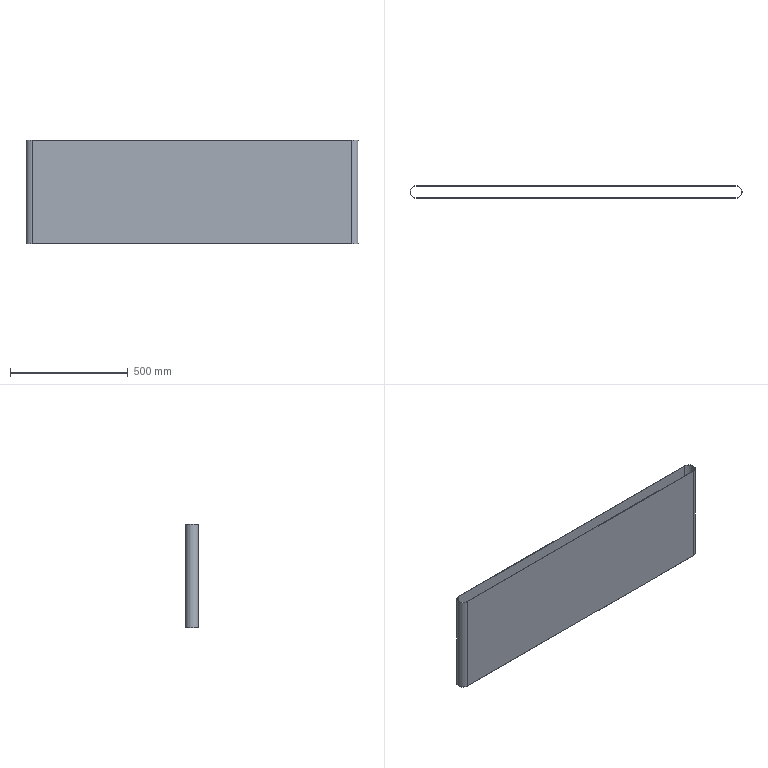Part | STEP file | RUBE 601 | 1 solid | 10 faces | box 1411 x 53.2 x 440 mm | volume 2026187 mm3 | plane 6 | cylinder 4 | commonest cylinder face diameters 50 x2 53.2 x2
STEP:
#1=CARTESIAN_POINT('',(0.,0.,0.));
#2=DIRECTION('',(0.,0.,1.));
#3=DIRECTION('',(1.,0.,0.));
#4=AXIS2_PLACEMENT_3D('',#1,#2,#3);
#5=CARTESIAN_POINT('',(-1248.5,28.6,220.));
#6=VERTEX_POINT('',#5);
#7=CARTESIAN_POINT('',(-1248.5,-24.6,220.));
#8=VERTEX_POINT('',#7);
#9=CARTESIAN_POINT('',(-1248.5,2.,220.));
#10=DIRECTION('',(0.,0.,1.));
#11=DIRECTION('',(1.,0.,0.));
#12=AXIS2_PLACEMENT_3D('',#9,#10,#11);
#13=CIRCLE('',#12,26.6);
#14=CARTESIAN_POINT('',(-1248.5,2.,220.));
#15=DIRECTION('',(0.,0.,1.));
#16=DIRECTION('',(1.,0.,0.));
#17=AXIS2_PLACEMENT_3D('',#14,#15,#16);
#18=PLANE('',#17);
#19=CARTESIAN_POINT('',(0.,0.));
#20=DIRECTION('',(1.,0.));
#21=AXIS2_PLACEMENT_2D('',#19,#20);
#22=CIRCLE('',#21,26.6);
#23=(GEOMETRIC_REPRESENTATION_CONTEXT(2)PARAMETRIC_REPRESENTATION_CONTEXT()REPRESENTATION_CONTEXT('',''));
#24=DEFINITIONAL_REPRESENTATION('',(#22),#23);
#25=PCURVE('',#18,#24);
#26=CARTESIAN_POINT('',(-1248.5,2.,220.));
#27=DIRECTION('',(0.,0.,-1.));
#28=DIRECTION('',(-1.,0.,0.));
#29=AXIS2_PLACEMENT_3D('',#26,#27,#28);
#30=CYLINDRICAL_SURFACE('',#29,26.6);
#31=CARTESIAN_POINT('',(3.142,0.));
#32=DIRECTION('',(-1.,0.));
#33=VECTOR('',#32,1.);
#34=LINE('',#31,#33);
#35=(GEOMETRIC_REPRESENTATION_CONTEXT(2)PARAMETRIC_REPRESENTATION_CONTEXT()REPRESENTATION_CONTEXT('',''));
#36=DEFINITIONAL_REPRESENTATION('',(#34),#35);
#37=PCURVE('',#30,#36);
#38=SURFACE_CURVE('',#13,(#25,#37),.PCURVE_S1.);
#39=EDGE_CURVE('',#6,#8,#38,.T.);
#40=ORIENTED_EDGE('',*,*,#39,.T.);
#41=CARTESIAN_POINT('',(109.5,-24.6,220.));
#42=VERTEX_POINT('',#41);
#43=CARTESIAN_POINT('',(-1248.5,-24.6,220.));
#44=DIRECTION('',(1.,0.,0.));
#45=VECTOR('',#44,1.);
#46=LINE('',#43,#45);
#47=CARTESIAN_POINT('',(0.,-26.6));
#48=DIRECTION('',(1.,0.));
#49=VECTOR('',#48,1.);
#50=LINE('',#47,#49);
#51=(GEOMETRIC_REPRESENTATION_CONTEXT(2)PARAMETRIC_REPRESENTATION_CONTEXT()REPRESENTATION_CONTEXT('',''));
#52=DEFINITIONAL_REPRESENTATION('',(#50),#51);
#53=PCURVE('',#18,#52);
#54=CARTESIAN_POINT('',(-1248.5,-24.6,220.));
#55=DIRECTION('',(0.,1.,0.));
#56=DIRECTION('',(-1.,0.,0.));
#57=AXIS2_PLACEMENT_3D('',#54,#55,#56);
#58=PLANE('',#57);
#59=CARTESIAN_POINT('',(0.,0.));
#60=DIRECTION('',(-1.,0.));
#61=VECTOR('',#60,1.);
#62=LINE('',#59,#61);
#63=(GEOMETRIC_REPRESENTATION_CONTEXT(2)PARAMETRIC_REPRESENTATION_CONTEXT()REPRESENTATION_CONTEXT('',''));
#64=DEFINITIONAL_REPRESENTATION('',(#62),#63);
#65=PCURVE('',#58,#64);
#66=SURFACE_CURVE('',#46,(#53,#65),.PCURVE_S1.);
#67=EDGE_CURVE('',#8,#42,#66,.T.);
#68=ORIENTED_EDGE('',*,*,#67,.T.);
#69=CARTESIAN_POINT('',(109.5,28.6,220.));
#70=VERTEX_POINT('',#69);
#71=CARTESIAN_POINT('',(109.5,2.,220.));
#72=DIRECTION('',(0.,0.,1.));
#73=DIRECTION('',(1.,0.,0.));
#74=AXIS2_PLACEMENT_3D('',#71,#72,#73);
#75=CIRCLE('',#74,26.6);
#76=CARTESIAN_POINT('',(1358.,0.));
#77=DIRECTION('',(1.,0.));
#78=AXIS2_PLACEMENT_2D('',#76,#77);
#79=CIRCLE('',#78,26.6);
#80=(GEOMETRIC_REPRESENTATION_CONTEXT(2)PARAMETRIC_REPRESENTATION_CONTEXT()REPRESENTATION_CONTEXT('',''));
#81=DEFINITIONAL_REPRESENTATION('',(#79),#80);
#82=PCURVE('',#18,#81);
#83=CARTESIAN_POINT('',(109.5,2.,220.));
#84=DIRECTION('',(0.,0.,-1.));
#85=DIRECTION('',(-1.,0.,0.));
#86=AXIS2_PLACEMENT_3D('',#83,#84,#85);
#87=CYLINDRICAL_SURFACE('',#86,26.6);
#88=CARTESIAN_POINT('',(9.425,0.));
#89=DIRECTION('',(-1.,0.));
#90=VECTOR('',#89,1.);
#91=LINE('',#88,#90);
#92=(GEOMETRIC_REPRESENTATION_CONTEXT(2)PARAMETRIC_REPRESENTATION_CONTEXT()REPRESENTATION_CONTEXT('',''));
#93=DEFINITIONAL_REPRESENTATION('',(#91),#92);
#94=PCURVE('',#87,#93);
#95=SURFACE_CURVE('',#75,(#82,#94),.PCURVE_S1.);
#96=EDGE_CURVE('',#42,#70,#95,.T.);
#97=ORIENTED_EDGE('',*,*,#96,.T.);
#98=CARTESIAN_POINT('',(-1248.5,28.6,220.));
#99=DIRECTION('',(-1.,0.,0.));
#100=VECTOR('',#99,1.);
#101=LINE('',#98,#100);
#102=CARTESIAN_POINT('',(0.,26.6));
#103=DIRECTION('',(-1.,0.));
#104=VECTOR('',#103,1.);
#105=LINE('',#102,#104);
#106=(GEOMETRIC_REPRESENTATION_CONTEXT(2)PARAMETRIC_REPRESENTATION_CONTEXT()REPRESENTATION_CONTEXT('',''));
#107=DEFINITIONAL_REPRESENTATION('',(#105),#106);
#108=PCURVE('',#18,#107);
#109=CARTESIAN_POINT('',(-1248.5,28.6,220.));
#110=DIRECTION('',(0.,-1.,0.));
#111=DIRECTION('',(1.,0.,0.));
#112=AXIS2_PLACEMENT_3D('',#109,#110,#111);
#113=PLANE('',#112);
#114=CARTESIAN_POINT('',(0.,0.));
#115=DIRECTION('',(-1.,0.));
#116=VECTOR('',#115,1.);
#117=LINE('',#114,#116);
#118=(GEOMETRIC_REPRESENTATION_CONTEXT(2)PARAMETRIC_REPRESENTATION_CONTEXT()REPRESENTATION_CONTEXT('',''));
#119=DEFINITIONAL_REPRESENTATION('',(#117),#118);
#120=PCURVE('',#113,#119);
#121=SURFACE_CURVE('',#101,(#108,#120),.PCURVE_S1.);
#122=EDGE_CURVE('',#70,#6,#121,.T.);
#123=ORIENTED_EDGE('',*,*,#122,.T.);
#124=EDGE_LOOP('',(#40,#68,#97,#123));
#125=FACE_BOUND('',#124,.T.);
#126=CARTESIAN_POINT('',(-1248.5,-23.,220.));
#127=VERTEX_POINT('',#126);
#128=CARTESIAN_POINT('',(109.5,-23.,220.));
#129=VERTEX_POINT('',#128);
#130=CARTESIAN_POINT('',(-1248.5,-23.,220.));
#131=DIRECTION('',(1.,0.,0.));
#132=VECTOR('',#131,1.);
#133=LINE('',#130,#132);
#134=CARTESIAN_POINT('',(0.,-25.));
#135=DIRECTION('',(1.,0.));
#136=VECTOR('',#135,1.);
#137=LINE('',#134,#136);
#138=(GEOMETRIC_REPRESENTATION_CONTEXT(2)PARAMETRIC_REPRESENTATION_CONTEXT()REPRESENTATION_CONTEXT('',''));
#139=DEFINITIONAL_REPRESENTATION('',(#137),#138);
#140=PCURVE('',#18,#139);
#141=CARTESIAN_POINT('',(-1248.5,-23.,220.));
#142=DIRECTION('',(0.,1.,0.));
#143=DIRECTION('',(-1.,0.,0.));
#144=AXIS2_PLACEMENT_3D('',#141,#142,#143);
#145=PLANE('',#144);
#146=CARTESIAN_POINT('',(0.,0.));
#147=DIRECTION('',(-1.,0.));
#148=VECTOR('',#147,1.);
#149=LINE('',#146,#148);
#150=(GEOMETRIC_REPRESENTATION_CONTEXT(2)PARAMETRIC_REPRESENTATION_CONTEXT()REPRESENTATION_CONTEXT('',''));
#151=DEFINITIONAL_REPRESENTATION('',(#149),#150);
#152=PCURVE('',#145,#151);
#153=SURFACE_CURVE('',#133,(#140,#152),.PCURVE_S1.);
#154=EDGE_CURVE('',#127,#129,#153,.T.);
#155=ORIENTED_EDGE('',*,*,#154,.F.);
#156=CARTESIAN_POINT('',(-1248.5,27.,220.));
#157=VERTEX_POINT('',#156);
#158=CARTESIAN_POINT('',(-1248.5,2.,220.));
#159=DIRECTION('',(0.,0.,1.));
#160=DIRECTION('',(1.,0.,0.));
#161=AXIS2_PLACEMENT_3D('',#158,#159,#160);
#162=CIRCLE('',#161,25.);
#163=CARTESIAN_POINT('',(0.,0.));
#164=DIRECTION('',(1.,0.));
#165=AXIS2_PLACEMENT_2D('',#163,#164);
#166=CIRCLE('',#165,25.);
#167=(GEOMETRIC_REPRESENTATION_CONTEXT(2)PARAMETRIC_REPRESENTATION_CONTEXT()REPRESENTATION_CONTEXT('',''));
#168=DEFINITIONAL_REPRESENTATION('',(#166),#167);
#169=PCURVE('',#18,#168);
#170=CARTESIAN_POINT('',(-1248.5,2.,220.));
#171=DIRECTION('',(0.,0.,-1.));
#172=DIRECTION('',(-1.,0.,0.));
#173=AXIS2_PLACEMENT_3D('',#170,#171,#172);
#174=CYLINDRICAL_SURFACE('',#173,25.);
#175=CARTESIAN_POINT('',(9.425,0.));
#176=DIRECTION('',(-1.,0.));
#177=VECTOR('',#176,1.);
#178=LINE('',#175,#177);
#179=(GEOMETRIC_REPRESENTATION_CONTEXT(2)PARAMETRIC_REPRESENTATION_CONTEXT()REPRESENTATION_CONTEXT('',''));
#180=DEFINITIONAL_REPRESENTATION('',(#178),#179);
#181=PCURVE('',#174,#180);
#182=SURFACE_CURVE('',#162,(#169,#181),.PCURVE_S1.);
#183=EDGE_CURVE('',#157,#127,#182,.T.);
#184=ORIENTED_EDGE('',*,*,#183,.F.);
#185=CARTESIAN_POINT('',(109.5,27.,220.));
#186=VERTEX_POINT('',#185);
#187=CARTESIAN_POINT('',(-1248.5,27.,220.));
#188=DIRECTION('',(-1.,0.,0.));
#189=VECTOR('',#188,1.);
#190=LINE('',#187,#189);
#191=CARTESIAN_POINT('',(0.,25.));
#192=DIRECTION('',(-1.,0.));
#193=VECTOR('',#192,1.);
#194=LINE('',#191,#193);
#195=(GEOMETRIC_REPRESENTATION_CONTEXT(2)PARAMETRIC_REPRESENTATION_CONTEXT()REPRESENTATION_CONTEXT('',''));
#196=DEFINITIONAL_REPRESENTATION('',(#194),#195);
#197=PCURVE('',#18,#196);
#198=CARTESIAN_POINT('',(-1248.5,27.,220.));
#199=DIRECTION('',(0.,-1.,0.));
#200=DIRECTION('',(1.,0.,0.));
#201=AXIS2_PLACEMENT_3D('',#198,#199,#200);
#202=PLANE('',#201);
#203=CARTESIAN_POINT('',(0.,0.));
#204=DIRECTION('',(-1.,0.));
#205=VECTOR('',#204,1.);
#206=LINE('',#203,#205);
#207=(GEOMETRIC_REPRESENTATION_CONTEXT(2)PARAMETRIC_REPRESENTATION_CONTEXT()REPRESENTATION_CONTEXT('',''));
#208=DEFINITIONAL_REPRESENTATION('',(#206),#207);
#209=PCURVE('',#202,#208);
#210=SURFACE_CURVE('',#190,(#197,#209),.PCURVE_S1.);
#211=EDGE_CURVE('',#186,#157,#210,.T.);
#212=ORIENTED_EDGE('',*,*,#211,.F.);
#213=CARTESIAN_POINT('',(109.5,2.,220.));
#214=DIRECTION('',(0.,0.,1.));
#215=DIRECTION('',(1.,0.,0.));
#216=AXIS2_PLACEMENT_3D('',#213,#214,#215);
#217=CIRCLE('',#216,25.);
#218=CARTESIAN_POINT('',(1358.,0.));
#219=DIRECTION('',(1.,0.));
#220=AXIS2_PLACEMENT_2D('',#218,#219);
#221=CIRCLE('',#220,25.);
#222=(GEOMETRIC_REPRESENTATION_CONTEXT(2)PARAMETRIC_REPRESENTATION_CONTEXT()REPRESENTATION_CONTEXT('',''));
#223=DEFINITIONAL_REPRESENTATION('',(#221),#222);
#224=PCURVE('',#18,#223);
#225=CARTESIAN_POINT('',(109.5,2.,220.));
#226=DIRECTION('',(0.,0.,-1.));
#227=DIRECTION('',(-1.,0.,0.));
#228=AXIS2_PLACEMENT_3D('',#225,#226,#227);
#229=CYLINDRICAL_SURFACE('',#228,25.);
#230=CARTESIAN_POINT('',(9.425,0.));
#231=DIRECTION('',(-1.,0.));
#232=VECTOR('',#231,1.);
#233=LINE('',#230,#232);
#234=(GEOMETRIC_REPRESENTATION_CONTEXT(2)PARAMETRIC_REPRESENTATION_CONTEXT()REPRESENTATION_CONTEXT('',''));
#235=DEFINITIONAL_REPRESENTATION('',(#233),#234);
#236=PCURVE('',#229,#235);
#237=SURFACE_CURVE('',#217,(#224,#236),.PCURVE_S1.);
#238=EDGE_CURVE('',#129,#186,#237,.T.);
#239=ORIENTED_EDGE('',*,*,#238,.F.);
#240=EDGE_LOOP('',(#155,#184,#212,#239));
#241=FACE_BOUND('',#240,.T.);
#242=ADVANCED_FACE('',(#125,#241),#18,.T.);
#243=CARTESIAN_POINT('',(-1248.5,28.6,-220.));
#244=VERTEX_POINT('',#243);
#245=CARTESIAN_POINT('',(-1248.5,-24.6,-220.));
#246=VERTEX_POINT('',#245);
#247=CARTESIAN_POINT('',(-1248.5,2.,-220.));
#248=DIRECTION('',(0.,0.,1.));
#249=DIRECTION('',(1.,0.,0.));
#250=AXIS2_PLACEMENT_3D('',#247,#248,#249);
#251=CIRCLE('',#250,26.6);
#252=CARTESIAN_POINT('',(-1248.5,2.,-220.));
#253=DIRECTION('',(0.,0.,1.));
#254=DIRECTION('',(1.,0.,0.));
#255=AXIS2_PLACEMENT_3D('',#252,#253,#254);
#256=PLANE('',#255);
#257=CARTESIAN_POINT('',(0.,0.));
#258=DIRECTION('',(1.,0.));
#259=AXIS2_PLACEMENT_2D('',#257,#258);
#260=CIRCLE('',#259,26.6);
#261=(GEOMETRIC_REPRESENTATION_CONTEXT(2)PARAMETRIC_REPRESENTATION_CONTEXT()REPRESENTATION_CONTEXT('',''));
#262=DEFINITIONAL_REPRESENTATION('',(#260),#261);
#263=PCURVE('',#256,#262);
#264=CARTESIAN_POINT('',(3.142,440.));
#265=DIRECTION('',(-1.,0.));
#266=VECTOR('',#265,1.);
#267=LINE('',#264,#266);
#268=(GEOMETRIC_REPRESENTATION_CONTEXT(2)PARAMETRIC_REPRESENTATION_CONTEXT()REPRESENTATION_CONTEXT('',''));
#269=DEFINITIONAL_REPRESENTATION('',(#267),#268);
#270=PCURVE('',#30,#269);
#271=SURFACE_CURVE('',#251,(#263,#270),.PCURVE_S1.);
#272=EDGE_CURVE('',#244,#246,#271,.T.);
#273=ORIENTED_EDGE('',*,*,#272,.F.);
#274=CARTESIAN_POINT('',(109.5,28.6,-220.));
#275=VERTEX_POINT('',#274);
#276=CARTESIAN_POINT('',(-1248.5,28.6,-220.));
#277=DIRECTION('',(-1.,0.,0.));
#278=VECTOR('',#277,1.);
#279=LINE('',#276,#278);
#280=CARTESIAN_POINT('',(0.,26.6));
#281=DIRECTION('',(-1.,0.));
#282=VECTOR('',#281,1.);
#283=LINE('',#280,#282);
#284=(GEOMETRIC_REPRESENTATION_CONTEXT(2)PARAMETRIC_REPRESENTATION_CONTEXT()REPRESENTATION_CONTEXT('',''));
#285=DEFINITIONAL_REPRESENTATION('',(#283),#284);
#286=PCURVE('',#256,#285);
#287=CARTESIAN_POINT('',(0.,-440.));
#288=DIRECTION('',(-1.,0.));
#289=VECTOR('',#288,1.);
#290=LINE('',#287,#289);
#291=(GEOMETRIC_REPRESENTATION_CONTEXT(2)PARAMETRIC_REPRESENTATION_CONTEXT()REPRESENTATION_CONTEXT('',''));
#292=DEFINITIONAL_REPRESENTATION('',(#290),#291);
#293=PCURVE('',#113,#292);
#294=SURFACE_CURVE('',#279,(#286,#293),.PCURVE_S1.);
#295=EDGE_CURVE('',#275,#244,#294,.T.);
#296=ORIENTED_EDGE('',*,*,#295,.F.);
#297=CARTESIAN_POINT('',(109.5,-24.6,-220.));
#298=VERTEX_POINT('',#297);
#299=CARTESIAN_POINT('',(109.5,2.,-220.));
#300=DIRECTION('',(0.,0.,1.));
#301=DIRECTION('',(1.,0.,0.));
#302=AXIS2_PLACEMENT_3D('',#299,#300,#301);
#303=CIRCLE('',#302,26.6);
#304=CARTESIAN_POINT('',(1358.,0.));
#305=DIRECTION('',(1.,0.));
#306=AXIS2_PLACEMENT_2D('',#304,#305);
#307=CIRCLE('',#306,26.6);
#308=(GEOMETRIC_REPRESENTATION_CONTEXT(2)PARAMETRIC_REPRESENTATION_CONTEXT()REPRESENTATION_CONTEXT('',''));
#309=DEFINITIONAL_REPRESENTATION('',(#307),#308);
#310=PCURVE('',#256,#309);
#311=CARTESIAN_POINT('',(9.425,440.));
#312=DIRECTION('',(-1.,0.));
#313=VECTOR('',#312,1.);
#314=LINE('',#311,#313);
#315=(GEOMETRIC_REPRESENTATION_CONTEXT(2)PARAMETRIC_REPRESENTATION_CONTEXT()REPRESENTATION_CONTEXT('',''));
#316=DEFINITIONAL_REPRESENTATION('',(#314),#315);
#317=PCURVE('',#87,#316);
#318=SURFACE_CURVE('',#303,(#310,#317),.PCURVE_S1.);
#319=EDGE_CURVE('',#298,#275,#318,.T.);
#320=ORIENTED_EDGE('',*,*,#319,.F.);
#321=CARTESIAN_POINT('',(-1248.5,-24.6,-220.));
#322=DIRECTION('',(1.,0.,0.));
#323=VECTOR('',#322,1.);
#324=LINE('',#321,#323);
#325=CARTESIAN_POINT('',(0.,-26.6));
#326=DIRECTION('',(1.,0.));
#327=VECTOR('',#326,1.);
#328=LINE('',#325,#327);
#329=(GEOMETRIC_REPRESENTATION_CONTEXT(2)PARAMETRIC_REPRESENTATION_CONTEXT()REPRESENTATION_CONTEXT('',''));
#330=DEFINITIONAL_REPRESENTATION('',(#328),#329);
#331=PCURVE('',#256,#330);
#332=CARTESIAN_POINT('',(0.,-440.));
#333=DIRECTION('',(-1.,0.));
#334=VECTOR('',#333,1.);
#335=LINE('',#332,#334);
#336=(GEOMETRIC_REPRESENTATION_CONTEXT(2)PARAMETRIC_REPRESENTATION_CONTEXT()REPRESENTATION_CONTEXT('',''));
#337=DEFINITIONAL_REPRESENTATION('',(#335),#336);
#338=PCURVE('',#58,#337);
#339=SURFACE_CURVE('',#324,(#331,#338),.PCURVE_S1.);
#340=EDGE_CURVE('',#246,#298,#339,.T.);
#341=ORIENTED_EDGE('',*,*,#340,.F.);
#342=EDGE_LOOP('',(#273,#296,#320,#341));
#343=FACE_BOUND('',#342,.T.);
#344=CARTESIAN_POINT('',(-1248.5,27.,-220.));
#345=VERTEX_POINT('',#344);
#346=CARTESIAN_POINT('',(-1248.5,-23.,-220.));
#347=VERTEX_POINT('',#346);
#348=CARTESIAN_POINT('',(-1248.5,2.,-220.));
#349=DIRECTION('',(0.,0.,1.));
#350=DIRECTION('',(1.,0.,0.));
#351=AXIS2_PLACEMENT_3D('',#348,#349,#350);
#352=CIRCLE('',#351,25.);
#353=CARTESIAN_POINT('',(0.,0.));
#354=DIRECTION('',(1.,0.));
#355=AXIS2_PLACEMENT_2D('',#353,#354);
#356=CIRCLE('',#355,25.);
#357=(GEOMETRIC_REPRESENTATION_CONTEXT(2)PARAMETRIC_REPRESENTATION_CONTEXT()REPRESENTATION_CONTEXT('',''));
#358=DEFINITIONAL_REPRESENTATION('',(#356),#357);
#359=PCURVE('',#256,#358);
#360=CARTESIAN_POINT('',(9.425,440.));
#361=DIRECTION('',(-1.,0.));
#362=VECTOR('',#361,1.);
#363=LINE('',#360,#362);
#364=(GEOMETRIC_REPRESENTATION_CONTEXT(2)PARAMETRIC_REPRESENTATION_CONTEXT()REPRESENTATION_CONTEXT('',''));
#365=DEFINITIONAL_REPRESENTATION('',(#363),#364);
#366=PCURVE('',#174,#365);
#367=SURFACE_CURVE('',#352,(#359,#366),.PCURVE_S1.);
#368=EDGE_CURVE('',#345,#347,#367,.T.);
#369=ORIENTED_EDGE('',*,*,#368,.T.);
#370=CARTESIAN_POINT('',(109.5,-23.,-220.));
#371=VERTEX_POINT('',#370);
#372=CARTESIAN_POINT('',(-1248.5,-23.,-220.));
#373=DIRECTION('',(1.,0.,0.));
#374=VECTOR('',#373,1.);
#375=LINE('',#372,#374);
#376=CARTESIAN_POINT('',(0.,-25.));
#377=DIRECTION('',(1.,0.));
#378=VECTOR('',#377,1.);
#379=LINE('',#376,#378);
#380=(GEOMETRIC_REPRESENTATION_CONTEXT(2)PARAMETRIC_REPRESENTATION_CONTEXT()REPRESENTATION_CONTEXT('',''));
#381=DEFINITIONAL_REPRESENTATION('',(#379),#380);
#382=PCURVE('',#256,#381);
#383=CARTESIAN_POINT('',(0.,-440.));
#384=DIRECTION('',(-1.,0.));
#385=VECTOR('',#384,1.);
#386=LINE('',#383,#385);
#387=(GEOMETRIC_REPRESENTATION_CONTEXT(2)PARAMETRIC_REPRESENTATION_CONTEXT()REPRESENTATION_CONTEXT('',''));
#388=DEFINITIONAL_REPRESENTATION('',(#386),#387);
#389=PCURVE('',#145,#388);
#390=SURFACE_CURVE('',#375,(#382,#389),.PCURVE_S1.);
#391=EDGE_CURVE('',#347,#371,#390,.T.);
#392=ORIENTED_EDGE('',*,*,#391,.T.);
#393=CARTESIAN_POINT('',(109.5,27.,-220.));
#394=VERTEX_POINT('',#393);
#395=CARTESIAN_POINT('',(109.5,2.,-220.));
#396=DIRECTION('',(0.,0.,1.));
#397=DIRECTION('',(1.,0.,0.));
#398=AXIS2_PLACEMENT_3D('',#395,#396,#397);
#399=CIRCLE('',#398,25.);
#400=CARTESIAN_POINT('',(1358.,0.));
#401=DIRECTION('',(1.,0.));
#402=AXIS2_PLACEMENT_2D('',#400,#401);
#403=CIRCLE('',#402,25.);
#404=(GEOMETRIC_REPRESENTATION_CONTEXT(2)PARAMETRIC_REPRESENTATION_CONTEXT()REPRESENTATION_CONTEXT('',''));
#405=DEFINITIONAL_REPRESENTATION('',(#403),#404);
#406=PCURVE('',#256,#405);
#407=CARTESIAN_POINT('',(9.425,440.));
#408=DIRECTION('',(-1.,0.));
#409=VECTOR('',#408,1.);
#410=LINE('',#407,#409);
#411=(GEOMETRIC_REPRESENTATION_CONTEXT(2)PARAMETRIC_REPRESENTATION_CONTEXT()REPRESENTATION_CONTEXT('',''));
#412=DEFINITIONAL_REPRESENTATION('',(#410),#411);
#413=PCURVE('',#229,#412);
#414=SURFACE_CURVE('',#399,(#406,#413),.PCURVE_S1.);
#415=EDGE_CURVE('',#371,#394,#414,.T.);
#416=ORIENTED_EDGE('',*,*,#415,.T.);
#417=CARTESIAN_POINT('',(-1248.5,27.,-220.));
#418=DIRECTION('',(-1.,0.,0.));
#419=VECTOR('',#418,1.);
#420=LINE('',#417,#419);
#421=CARTESIAN_POINT('',(0.,25.));
#422=DIRECTION('',(-1.,0.));
#423=VECTOR('',#422,1.);
#424=LINE('',#421,#423);
#425=(GEOMETRIC_REPRESENTATION_CONTEXT(2)PARAMETRIC_REPRESENTATION_CONTEXT()REPRESENTATION_CONTEXT('',''));
#426=DEFINITIONAL_REPRESENTATION('',(#424),#425);
#427=PCURVE('',#256,#426);
#428=CARTESIAN_POINT('',(0.,-440.));
#429=DIRECTION('',(-1.,0.));
#430=VECTOR('',#429,1.);
#431=LINE('',#428,#430);
#432=(GEOMETRIC_REPRESENTATION_CONTEXT(2)PARAMETRIC_REPRESENTATION_CONTEXT()REPRESENTATION_CONTEXT('',''));
#433=DEFINITIONAL_REPRESENTATION('',(#431),#432);
#434=PCURVE('',#202,#433);
#435=SURFACE_CURVE('',#420,(#427,#434),.PCURVE_S1.);
#436=EDGE_CURVE('',#394,#345,#435,.T.);
#437=ORIENTED_EDGE('',*,*,#436,.T.);
#438=EDGE_LOOP('',(#369,#392,#416,#437));
#439=FACE_BOUND('',#438,.T.);
#440=ADVANCED_FACE('',(#343,#439),#256,.F.);
#441=ORIENTED_EDGE('',*,*,#272,.T.);
#442=CARTESIAN_POINT('',(-1248.5,-24.6,220.));
#443=DIRECTION('',(0.,0.,-1.));
#444=VECTOR('',#443,1.);
#445=LINE('',#442,#444);
#446=CARTESIAN_POINT('',(-1.571,0.));
#447=DIRECTION('',(0.,1.));
#448=VECTOR('',#447,1.);
#449=LINE('',#446,#448);
#450=(GEOMETRIC_REPRESENTATION_CONTEXT(2)PARAMETRIC_REPRESENTATION_CONTEXT()REPRESENTATION_CONTEXT('',''));
#451=DEFINITIONAL_REPRESENTATION('',(#449),#450);
#452=PCURVE('',#30,#451);
#453=CARTESIAN_POINT('',(0.,0.));
#454=DIRECTION('',(0.,-1.));
#455=VECTOR('',#454,1.);
#456=LINE('',#453,#455);
#457=(GEOMETRIC_REPRESENTATION_CONTEXT(2)PARAMETRIC_REPRESENTATION_CONTEXT()REPRESENTATION_CONTEXT('',''));
#458=DEFINITIONAL_REPRESENTATION('',(#456),#457);
#459=PCURVE('',#58,#458);
#460=SURFACE_CURVE('',#445,(#452,#459),.PCURVE_S1.);
#461=EDGE_CURVE('',#8,#246,#460,.T.);
#462=ORIENTED_EDGE('',*,*,#461,.F.);
#463=ORIENTED_EDGE('',*,*,#39,.F.);
#464=CARTESIAN_POINT('',(-1248.5,28.6,220.));
#465=DIRECTION('',(0.,0.,-1.));
#466=VECTOR('',#465,1.);
#467=LINE('',#464,#466);
#468=CARTESIAN_POINT('',(1.571,0.));
#469=DIRECTION('',(0.,1.));
#470=VECTOR('',#469,1.);
#471=LINE('',#468,#470);
#472=(GEOMETRIC_REPRESENTATION_CONTEXT(2)PARAMETRIC_REPRESENTATION_CONTEXT()REPRESENTATION_CONTEXT('',''));
#473=DEFINITIONAL_REPRESENTATION('',(#471),#472);
#474=PCURVE('',#30,#473);
#475=CARTESIAN_POINT('',(0.,0.));
#476=DIRECTION('',(0.,-1.));
#477=VECTOR('',#476,1.);
#478=LINE('',#475,#477);
#479=(GEOMETRIC_REPRESENTATION_CONTEXT(2)PARAMETRIC_REPRESENTATION_CONTEXT()REPRESENTATION_CONTEXT('',''));
#480=DEFINITIONAL_REPRESENTATION('',(#478),#479);
#481=PCURVE('',#113,#480);
#482=SURFACE_CURVE('',#467,(#474,#481),.PCURVE_S1.);
#483=EDGE_CURVE('',#6,#244,#482,.T.);
#484=ORIENTED_EDGE('',*,*,#483,.T.);
#485=EDGE_LOOP('',(#441,#462,#463,#484));
#486=FACE_BOUND('',#485,.T.);
#487=ADVANCED_FACE('',(#486),#30,.T.);
#488=ORIENTED_EDGE('',*,*,#340,.T.);
#489=CARTESIAN_POINT('',(109.5,-24.6,220.));
#490=DIRECTION('',(0.,0.,-1.));
#491=VECTOR('',#490,1.);
#492=LINE('',#489,#491);
#493=CARTESIAN_POINT('',(-1358.,0.));
#494=DIRECTION('',(0.,-1.));
#495=VECTOR('',#494,1.);
#496=LINE('',#493,#495);
#497=(GEOMETRIC_REPRESENTATION_CONTEXT(2)PARAMETRIC_REPRESENTATION_CONTEXT()REPRESENTATION_CONTEXT('',''));
#498=DEFINITIONAL_REPRESENTATION('',(#496),#497);
#499=PCURVE('',#58,#498);
#500=CARTESIAN_POINT('',(4.712,0.));
#501=DIRECTION('',(0.,1.));
#502=VECTOR('',#501,1.);
#503=LINE('',#500,#502);
#504=(GEOMETRIC_REPRESENTATION_CONTEXT(2)PARAMETRIC_REPRESENTATION_CONTEXT()REPRESENTATION_CONTEXT('',''));
#505=DEFINITIONAL_REPRESENTATION('',(#503),#504);
#506=PCURVE('',#87,#505);
#507=SURFACE_CURVE('',#492,(#499,#506),.PCURVE_S1.);
#508=EDGE_CURVE('',#42,#298,#507,.T.);
#509=ORIENTED_EDGE('',*,*,#508,.F.);
#510=ORIENTED_EDGE('',*,*,#67,.F.);
#511=ORIENTED_EDGE('',*,*,#461,.T.);
#512=EDGE_LOOP('',(#488,#509,#510,#511));
#513=FACE_BOUND('',#512,.T.);
#514=ADVANCED_FACE('',(#513),#58,.F.);
#515=ORIENTED_EDGE('',*,*,#319,.T.);
#516=CARTESIAN_POINT('',(109.5,28.6,220.));
#517=DIRECTION('',(0.,0.,-1.));
#518=VECTOR('',#517,1.);
#519=LINE('',#516,#518);
#520=CARTESIAN_POINT('',(1.571,0.));
#521=DIRECTION('',(0.,1.));
#522=VECTOR('',#521,1.);
#523=LINE('',#520,#522);
#524=(GEOMETRIC_REPRESENTATION_CONTEXT(2)PARAMETRIC_REPRESENTATION_CONTEXT()REPRESENTATION_CONTEXT('',''));
#525=DEFINITIONAL_REPRESENTATION('',(#523),#524);
#526=PCURVE('',#87,#525);
#527=CARTESIAN_POINT('',(1358.,0.));
#528=DIRECTION('',(0.,-1.));
#529=VECTOR('',#528,1.);
#530=LINE('',#527,#529);
#531=(GEOMETRIC_REPRESENTATION_CONTEXT(2)PARAMETRIC_REPRESENTATION_CONTEXT()REPRESENTATION_CONTEXT('',''));
#532=DEFINITIONAL_REPRESENTATION('',(#530),#531);
#533=PCURVE('',#113,#532);
#534=SURFACE_CURVE('',#519,(#526,#533),.PCURVE_S1.);
#535=EDGE_CURVE('',#70,#275,#534,.T.);
#536=ORIENTED_EDGE('',*,*,#535,.F.);
#537=ORIENTED_EDGE('',*,*,#96,.F.);
#538=ORIENTED_EDGE('',*,*,#508,.T.);
#539=EDGE_LOOP('',(#515,#536,#537,#538));
#540=FACE_BOUND('',#539,.T.);
#541=ADVANCED_FACE('',(#540),#87,.T.);
#542=ORIENTED_EDGE('',*,*,#295,.T.);
#543=ORIENTED_EDGE('',*,*,#483,.F.);
#544=ORIENTED_EDGE('',*,*,#122,.F.);
#545=ORIENTED_EDGE('',*,*,#535,.T.);
#546=EDGE_LOOP('',(#542,#543,#544,#545));
#547=FACE_BOUND('',#546,.T.);
#548=ADVANCED_FACE('',(#547),#113,.F.);
#549=CARTESIAN_POINT('',(-1248.5,-23.,220.));
#550=DIRECTION('',(0.,0.,-1.));
#551=VECTOR('',#550,1.);
#552=LINE('',#549,#551);
#553=CARTESIAN_POINT('',(4.712,0.));
#554=DIRECTION('',(0.,1.));
#555=VECTOR('',#554,1.);
#556=LINE('',#553,#555);
#557=(GEOMETRIC_REPRESENTATION_CONTEXT(2)PARAMETRIC_REPRESENTATION_CONTEXT()REPRESENTATION_CONTEXT('',''));
#558=DEFINITIONAL_REPRESENTATION('',(#556),#557);
#559=PCURVE('',#174,#558);
#560=CARTESIAN_POINT('',(0.,0.));
#561=DIRECTION('',(0.,-1.));
#562=VECTOR('',#561,1.);
#563=LINE('',#560,#562);
#564=(GEOMETRIC_REPRESENTATION_CONTEXT(2)PARAMETRIC_REPRESENTATION_CONTEXT()REPRESENTATION_CONTEXT('',''));
#565=DEFINITIONAL_REPRESENTATION('',(#563),#564);
#566=PCURVE('',#145,#565);
#567=SURFACE_CURVE('',#552,(#559,#566),.PCURVE_S1.);
#568=EDGE_CURVE('',#127,#347,#567,.T.);
#569=ORIENTED_EDGE('',*,*,#568,.F.);
#570=ORIENTED_EDGE('',*,*,#183,.F.);
#571=CARTESIAN_POINT('',(-1248.5,27.,220.));
#572=DIRECTION('',(0.,0.,-1.));
#573=VECTOR('',#572,1.);
#574=LINE('',#571,#573);
#575=CARTESIAN_POINT('',(7.854,0.));
#576=DIRECTION('',(0.,1.));
#577=VECTOR('',#576,1.);
#578=LINE('',#575,#577);
#579=(GEOMETRIC_REPRESENTATION_CONTEXT(2)PARAMETRIC_REPRESENTATION_CONTEXT()REPRESENTATION_CONTEXT('',''));
#580=DEFINITIONAL_REPRESENTATION('',(#578),#579);
#581=PCURVE('',#174,#580);
#582=CARTESIAN_POINT('',(0.,0.));
#583=DIRECTION('',(0.,-1.));
#584=VECTOR('',#583,1.);
#585=LINE('',#582,#584);
#586=(GEOMETRIC_REPRESENTATION_CONTEXT(2)PARAMETRIC_REPRESENTATION_CONTEXT()REPRESENTATION_CONTEXT('',''));
#587=DEFINITIONAL_REPRESENTATION('',(#585),#586);
#588=PCURVE('',#202,#587);
#589=SURFACE_CURVE('',#574,(#581,#588),.PCURVE_S1.);
#590=EDGE_CURVE('',#157,#345,#589,.T.);
#591=ORIENTED_EDGE('',*,*,#590,.T.);
#592=ORIENTED_EDGE('',*,*,#368,.T.);
#593=EDGE_LOOP('',(#569,#570,#591,#592));
#594=FACE_BOUND('',#593,.F.);
#595=ADVANCED_FACE('',(#594),#174,.F.);
#596=ORIENTED_EDGE('',*,*,#391,.F.);
#597=ORIENTED_EDGE('',*,*,#568,.F.);
#598=ORIENTED_EDGE('',*,*,#154,.T.);
#599=CARTESIAN_POINT('',(109.5,-23.,220.));
#600=DIRECTION('',(0.,0.,-1.));
#601=VECTOR('',#600,1.);
#602=LINE('',#599,#601);
#603=CARTESIAN_POINT('',(-1358.,0.));
#604=DIRECTION('',(0.,-1.));
#605=VECTOR('',#604,1.);
#606=LINE('',#603,#605);
#607=(GEOMETRIC_REPRESENTATION_CONTEXT(2)PARAMETRIC_REPRESENTATION_CONTEXT()REPRESENTATION_CONTEXT('',''));
#608=DEFINITIONAL_REPRESENTATION('',(#606),#607);
#609=PCURVE('',#145,#608);
#610=CARTESIAN_POINT('',(4.712,0.));
#611=DIRECTION('',(0.,1.));
#612=VECTOR('',#611,1.);
#613=LINE('',#610,#612);
#614=(GEOMETRIC_REPRESENTATION_CONTEXT(2)PARAMETRIC_REPRESENTATION_CONTEXT()REPRESENTATION_CONTEXT('',''));
#615=DEFINITIONAL_REPRESENTATION('',(#613),#614);
#616=PCURVE('',#229,#615);
#617=SURFACE_CURVE('',#602,(#609,#616),.PCURVE_S1.);
#618=EDGE_CURVE('',#129,#371,#617,.T.);
#619=ORIENTED_EDGE('',*,*,#618,.T.);
#620=EDGE_LOOP('',(#596,#597,#598,#619));
#621=FACE_BOUND('',#620,.T.);
#622=ADVANCED_FACE('',(#621),#145,.T.);
#623=CARTESIAN_POINT('',(109.5,27.,220.));
#624=DIRECTION('',(0.,0.,-1.));
#625=VECTOR('',#624,1.);
#626=LINE('',#623,#625);
#627=CARTESIAN_POINT('',(1.571,0.));
#628=DIRECTION('',(0.,1.));
#629=VECTOR('',#628,1.);
#630=LINE('',#627,#629);
#631=(GEOMETRIC_REPRESENTATION_CONTEXT(2)PARAMETRIC_REPRESENTATION_CONTEXT()REPRESENTATION_CONTEXT('',''));
#632=DEFINITIONAL_REPRESENTATION('',(#630),#631);
#633=PCURVE('',#229,#632);
#634=CARTESIAN_POINT('',(1358.,0.));
#635=DIRECTION('',(0.,-1.));
#636=VECTOR('',#635,1.);
#637=LINE('',#634,#636);
#638=(GEOMETRIC_REPRESENTATION_CONTEXT(2)PARAMETRIC_REPRESENTATION_CONTEXT()REPRESENTATION_CONTEXT('',''));
#639=DEFINITIONAL_REPRESENTATION('',(#637),#638);
#640=PCURVE('',#202,#639);
#641=SURFACE_CURVE('',#626,(#633,#640),.PCURVE_S1.);
#642=EDGE_CURVE('',#186,#394,#641,.T.);
#643=ORIENTED_EDGE('',*,*,#642,.F.);
#644=ORIENTED_EDGE('',*,*,#238,.F.);
#645=ORIENTED_EDGE('',*,*,#618,.T.);
#646=ORIENTED_EDGE('',*,*,#415,.T.);
#647=EDGE_LOOP('',(#643,#644,#645,#646));
#648=FACE_BOUND('',#647,.F.);
#649=ADVANCED_FACE('',(#648),#229,.F.);
#650=ORIENTED_EDGE('',*,*,#436,.F.);
#651=ORIENTED_EDGE('',*,*,#642,.F.);
#652=ORIENTED_EDGE('',*,*,#211,.T.);
#653=ORIENTED_EDGE('',*,*,#590,.T.);
#654=EDGE_LOOP('',(#650,#651,#652,#653));
#655=FACE_BOUND('',#654,.T.);
#656=ADVANCED_FACE('',(#655),#202,.T.);
#657=CLOSED_SHELL('',(#242,#440,#487,#514,#541,#548,#595,#622,#649,#656));
#658=MANIFOLD_SOLID_BREP('',#657);
#659=(LENGTH_UNIT()NAMED_UNIT(*)SI_UNIT(.MILLI.,.METRE.));
#660=UNCERTAINTY_MEASURE_WITH_UNIT(LENGTH_MEASURE(0.0000001),#659,'','');
#661=(NAMED_UNIT(*)PLANE_ANGLE_UNIT()SI_UNIT($,.RADIAN.));
#662=(NAMED_UNIT(*)SI_UNIT($,.STERADIAN.)SOLID_ANGLE_UNIT());
#663=(GEOMETRIC_REPRESENTATION_CONTEXT(3)GLOBAL_UNCERTAINTY_ASSIGNED_CONTEXT((#660))GLOBAL_UNIT_ASSIGNED_CONTEXT((#659,#661,#662))REPRESENTATION_CONTEXT('',''));
#664=ADVANCED_BREP_SHAPE_REPRESENTATION('',(#4,#658),#663);